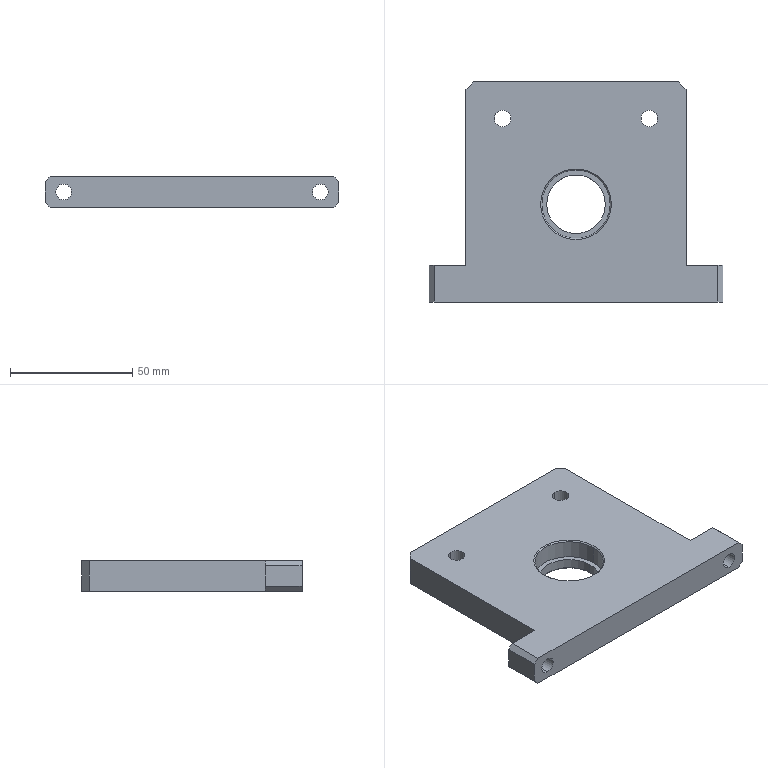Part | SolidWorks | features ICE 4, Chamfer 3, HoleWzd 2, Extrusion 1 | 1 solid | 33 faces | box 120 x 90 x 12.5 mm | volume 97757 mm3 | plane 17 | cylinder 12 | cone 4 | commonest cylinder face diameters 6.5 x4 6.8 x4 24 x2 28 x2
STEP:
#1=CARTESIAN_POINT('',(97.5,0.,-9.5));
#2=VERTEX_POINT('',#1);
#3=CARTESIAN_POINT('',(97.5,0.,-3.));
#4=VERTEX_POINT('',#3);
#5=CARTESIAN_POINT('',(97.5,0.,-6.25));
#6=DIRECTION('',(0.,1.,0.));
#7=DIRECTION('',(0.,0.,1.));
#8=AXIS2_PLACEMENT_3D('',#5,#6,#7);
#9=CIRCLE('',#8,3.25);
#10=EDGE_CURVE('',#2,#4,#9,.T.);
#11=ORIENTED_EDGE('',*,*,#10,.F.);
#12=CARTESIAN_POINT('',(97.5,15.,-9.5));
#13=VERTEX_POINT('',#12);
#14=CARTESIAN_POINT('',(97.5,15.,-9.5));
#15=DIRECTION('',(0.,1.,0.));
#16=VECTOR('',#15,1000.);
#17=LINE('',#14,#16);
#18=EDGE_CURVE('',#2,#13,#17,.T.);
#19=ORIENTED_EDGE('',*,*,#18,.T.);
#20=CARTESIAN_POINT('',(97.5,15.,-3.));
#21=VERTEX_POINT('',#20);
#22=CARTESIAN_POINT('',(97.5,15.,-6.25));
#23=DIRECTION('',(0.,1.,0.));
#24=DIRECTION('',(0.,0.,1.));
#25=AXIS2_PLACEMENT_3D('',#22,#23,#24);
#26=CIRCLE('',#25,3.25);
#27=EDGE_CURVE('',#13,#21,#26,.T.);
#28=ORIENTED_EDGE('',*,*,#27,.T.);
#29=CARTESIAN_POINT('',(97.5,15.,-3.));
#30=DIRECTION('',(0.,1.,0.));
#31=VECTOR('',#30,1000.);
#32=LINE('',#29,#31);
#33=EDGE_CURVE('',#4,#21,#32,.T.);
#34=ORIENTED_EDGE('',*,*,#33,.F.);
#35=EDGE_LOOP('',(#11,#19,#28,#34));
#36=FACE_OUTER_BOUND('',#35,.T.);
#37=CARTESIAN_POINT('',(97.5,15.,-6.25));
#38=DIRECTION('',(0.,1.,0.));
#39=DIRECTION('',(0.,0.,1.));
#40=AXIS2_PLACEMENT_3D('',#37,#38,#39);
#41=CYLINDRICAL_SURFACE('',#40,3.25);
#42=ADVANCED_FACE('',(#36),#41,.F.);
#43=CARTESIAN_POINT('',(-7.5,0.,-9.5));
#44=VERTEX_POINT('',#43);
#45=CARTESIAN_POINT('',(-7.5,0.,-3.));
#46=VERTEX_POINT('',#45);
#47=CARTESIAN_POINT('',(-7.5,0.,-6.25));
#48=DIRECTION('',(0.,1.,0.));
#49=DIRECTION('',(0.,0.,1.));
#50=AXIS2_PLACEMENT_3D('',#47,#48,#49);
#51=CIRCLE('',#50,3.25);
#52=EDGE_CURVE('',#44,#46,#51,.T.);
#53=ORIENTED_EDGE('',*,*,#52,.F.);
#54=CARTESIAN_POINT('',(-7.5,15.,-9.5));
#55=VERTEX_POINT('',#54);
#56=CARTESIAN_POINT('',(-7.5,15.,-9.5));
#57=DIRECTION('',(0.,1.,0.));
#58=VECTOR('',#57,1000.);
#59=LINE('',#56,#58);
#60=EDGE_CURVE('',#44,#55,#59,.T.);
#61=ORIENTED_EDGE('',*,*,#60,.T.);
#62=CARTESIAN_POINT('',(-7.5,15.,-3.));
#63=VERTEX_POINT('',#62);
#64=CARTESIAN_POINT('',(-7.5,15.,-6.25));
#65=DIRECTION('',(0.,1.,0.));
#66=DIRECTION('',(0.,0.,1.));
#67=AXIS2_PLACEMENT_3D('',#64,#65,#66);
#68=CIRCLE('',#67,3.25);
#69=EDGE_CURVE('',#55,#63,#68,.T.);
#70=ORIENTED_EDGE('',*,*,#69,.T.);
#71=CARTESIAN_POINT('',(-7.5,15.,-3.));
#72=DIRECTION('',(0.,1.,0.));
#73=VECTOR('',#72,1000.);
#74=LINE('',#71,#73);
#75=EDGE_CURVE('',#46,#63,#74,.T.);
#76=ORIENTED_EDGE('',*,*,#75,.F.);
#77=EDGE_LOOP('',(#53,#61,#70,#76));
#78=FACE_OUTER_BOUND('',#77,.T.);
#79=CARTESIAN_POINT('',(-7.5,15.,-6.25));
#80=DIRECTION('',(0.,1.,0.));
#81=DIRECTION('',(0.,0.,1.));
#82=AXIS2_PLACEMENT_3D('',#79,#80,#81);
#83=CYLINDRICAL_SURFACE('',#82,3.25);
#84=ADVANCED_FACE('',(#78),#83,.F.);
#85=CARTESIAN_POINT('',(31.,40.,-0.5));
#86=VERTEX_POINT('',#85);
#87=CARTESIAN_POINT('',(59.,40.,-0.5));
#88=VERTEX_POINT('',#87);
#89=CARTESIAN_POINT('',(45.,40.,-0.5));
#90=DIRECTION('',(0.,0.,1.));
#91=DIRECTION('',(-1.,0.,0.));
#92=AXIS2_PLACEMENT_3D('',#89,#90,#91);
#93=CIRCLE('',#92,14.);
#94=EDGE_CURVE('',#86,#88,#93,.T.);
#95=ORIENTED_EDGE('',*,*,#94,.F.);
#96=CARTESIAN_POINT('',(30.5,40.,0.));
#97=VERTEX_POINT('',#96);
#98=CARTESIAN_POINT('',(31.,40.,-0.5));
#99=DIRECTION('',(-0.7071,0.,0.7071));
#100=VECTOR('',#99,1000.);
#101=LINE('',#98,#100);
#102=EDGE_CURVE('',#86,#97,#101,.T.);
#103=ORIENTED_EDGE('',*,*,#102,.T.);
#104=CARTESIAN_POINT('',(59.5,40.,0.));
#105=VERTEX_POINT('',#104);
#106=CARTESIAN_POINT('',(45.,40.,0.));
#107=DIRECTION('',(0.,0.,-1.));
#108=DIRECTION('',(-1.,0.,0.));
#109=AXIS2_PLACEMENT_3D('',#106,#107,#108);
#110=CIRCLE('',#109,14.5);
#111=EDGE_CURVE('',#105,#97,#110,.T.);
#112=ORIENTED_EDGE('',*,*,#111,.F.);
#113=CARTESIAN_POINT('',(59.,40.,-0.5));
#114=DIRECTION('',(0.7071,0.,0.7071));
#115=VECTOR('',#114,1000.);
#116=LINE('',#113,#115);
#117=EDGE_CURVE('',#88,#105,#116,.T.);
#118=ORIENTED_EDGE('',*,*,#117,.F.);
#119=EDGE_LOOP('',(#95,#103,#112,#118));
#120=FACE_OUTER_BOUND('',#119,.T.);
#121=CARTESIAN_POINT('',(45.,40.,-0.5));
#122=DIRECTION('',(0.,0.,1.));
#123=DIRECTION('',(1.,0.,0.));
#124=AXIS2_PLACEMENT_3D('',#121,#122,#123);
#125=CONICAL_SURFACE('',#124,14.,0.7854);
#126=ADVANCED_FACE('',(#120),#125,.F.);
#127=CARTESIAN_POINT('',(57.,40.,-12.));
#128=VERTEX_POINT('',#127);
#129=CARTESIAN_POINT('',(33.,40.,-12.));
#130=VERTEX_POINT('',#129);
#131=CARTESIAN_POINT('',(45.,40.,-12.));
#132=DIRECTION('',(0.,0.,-1.));
#133=DIRECTION('',(1.,0.,0.));
#134=AXIS2_PLACEMENT_3D('',#131,#132,#133);
#135=CIRCLE('',#134,12.);
#136=EDGE_CURVE('',#128,#130,#135,.T.);
#137=ORIENTED_EDGE('',*,*,#136,.F.);
#138=CARTESIAN_POINT('',(57.5,40.,-12.5));
#139=VERTEX_POINT('',#138);
#140=CARTESIAN_POINT('',(57.5,40.,-12.5));
#141=DIRECTION('',(0.7071,0.,-0.7071));
#142=VECTOR('',#141,1000.);
#143=LINE('',#140,#142);
#144=EDGE_CURVE('',#128,#139,#143,.T.);
#145=ORIENTED_EDGE('',*,*,#144,.T.);
#146=CARTESIAN_POINT('',(32.5,40.,-12.5));
#147=VERTEX_POINT('',#146);
#148=CARTESIAN_POINT('',(45.,40.,-12.5));
#149=DIRECTION('',(0.,0.,1.));
#150=DIRECTION('',(0.,-1.,0.));
#151=AXIS2_PLACEMENT_3D('',#148,#149,#150);
#152=CIRCLE('',#151,12.5);
#153=EDGE_CURVE('',#147,#139,#152,.T.);
#154=ORIENTED_EDGE('',*,*,#153,.F.);
#155=CARTESIAN_POINT('',(32.5,40.,-12.5));
#156=DIRECTION('',(-0.7071,0.,-0.7071));
#157=VECTOR('',#156,1000.);
#158=LINE('',#155,#157);
#159=EDGE_CURVE('',#130,#147,#158,.T.);
#160=ORIENTED_EDGE('',*,*,#159,.F.);
#161=EDGE_LOOP('',(#137,#145,#154,#160));
#162=FACE_OUTER_BOUND('',#161,.T.);
#163=CARTESIAN_POINT('',(45.,40.,-12.5));
#164=DIRECTION('',(0.,0.,-1.));
#165=DIRECTION('',(-1.,0.,0.));
#166=AXIS2_PLACEMENT_3D('',#163,#164,#165);
#167=CONICAL_SURFACE('',#166,12.5,0.7854);
#168=ADVANCED_FACE('',(#162),#167,.F.);
#169=ORIENTED_EDGE('',*,*,#136,.T.);
#170=CARTESIAN_POINT('',(33.,40.,-8.));
#171=VERTEX_POINT('',#170);
#172=CARTESIAN_POINT('',(33.,40.,-12.5));
#173=DIRECTION('',(0.,0.,1.));
#174=VECTOR('',#173,1000.);
#175=LINE('',#172,#174);
#176=EDGE_CURVE('',#130,#171,#175,.T.);
#177=ORIENTED_EDGE('',*,*,#176,.T.);
#178=CARTESIAN_POINT('',(57.,40.,-8.));
#179=VERTEX_POINT('',#178);
#180=CARTESIAN_POINT('',(45.,40.,-8.));
#181=DIRECTION('',(0.,0.,1.));
#182=DIRECTION('',(1.,0.,0.));
#183=AXIS2_PLACEMENT_3D('',#180,#181,#182);
#184=CIRCLE('',#183,12.);
#185=EDGE_CURVE('',#171,#179,#184,.T.);
#186=ORIENTED_EDGE('',*,*,#185,.T.);
#187=CARTESIAN_POINT('',(57.,40.,-12.5));
#188=DIRECTION('',(0.,0.,1.));
#189=VECTOR('',#188,1000.);
#190=LINE('',#187,#189);
#191=EDGE_CURVE('',#128,#179,#190,.T.);
#192=ORIENTED_EDGE('',*,*,#191,.F.);
#193=EDGE_LOOP('',(#169,#177,#186,#192));
#194=FACE_OUTER_BOUND('',#193,.T.);
#195=CARTESIAN_POINT('',(45.,40.,-12.5));
#196=DIRECTION('',(0.,0.,1.));
#197=DIRECTION('',(1.,0.,0.));
#198=AXIS2_PLACEMENT_3D('',#195,#196,#197);
#199=CYLINDRICAL_SURFACE('',#198,12.);
#200=ADVANCED_FACE('',(#194),#199,.F.);
#201=CARTESIAN_POINT('',(31.,40.,-8.));
#202=VERTEX_POINT('',#201);
#203=CARTESIAN_POINT('',(59.,40.,-8.));
#204=VERTEX_POINT('',#203);
#205=CARTESIAN_POINT('',(45.,40.,-8.));
#206=DIRECTION('',(0.,0.,1.));
#207=DIRECTION('',(1.,0.,0.));
#208=AXIS2_PLACEMENT_3D('',#205,#206,#207);
#209=CIRCLE('',#208,14.);
#210=EDGE_CURVE('',#202,#204,#209,.T.);
#211=ORIENTED_EDGE('',*,*,#210,.F.);
#212=CARTESIAN_POINT('',(31.,40.,-8.));
#213=DIRECTION('',(0.,0.,1.));
#214=VECTOR('',#213,1000.);
#215=LINE('',#212,#214);
#216=EDGE_CURVE('',#202,#86,#215,.T.);
#217=ORIENTED_EDGE('',*,*,#216,.T.);
#218=ORIENTED_EDGE('',*,*,#94,.T.);
#219=CARTESIAN_POINT('',(59.,40.,-8.));
#220=DIRECTION('',(0.,0.,1.));
#221=VECTOR('',#220,1000.);
#222=LINE('',#219,#221);
#223=EDGE_CURVE('',#204,#88,#222,.T.);
#224=ORIENTED_EDGE('',*,*,#223,.F.);
#225=EDGE_LOOP('',(#211,#217,#218,#224));
#226=FACE_OUTER_BOUND('',#225,.T.);
#227=CARTESIAN_POINT('',(45.,40.,-8.));
#228=DIRECTION('',(0.,0.,1.));
#229=DIRECTION('',(1.,0.,0.));
#230=AXIS2_PLACEMENT_3D('',#227,#228,#229);
#231=CYLINDRICAL_SURFACE('',#230,14.);
#232=ADVANCED_FACE('',(#226),#231,.F.);
#233=CARTESIAN_POINT('',(15.,71.6,0.));
#234=VERTEX_POINT('',#233);
#235=CARTESIAN_POINT('',(15.,78.4,0.));
#236=VERTEX_POINT('',#235);
#237=CARTESIAN_POINT('',(15.,75.,0.));
#238=DIRECTION('',(0.,0.,-1.));
#239=DIRECTION('',(0.,1.,0.));
#240=AXIS2_PLACEMENT_3D('',#237,#238,#239);
#241=CIRCLE('',#240,3.4);
#242=EDGE_CURVE('',#234,#236,#241,.T.);
#243=ORIENTED_EDGE('',*,*,#242,.F.);
#244=CARTESIAN_POINT('',(15.,71.6,-12.5));
#245=VERTEX_POINT('',#244);
#246=CARTESIAN_POINT('',(15.,71.6,-12.5));
#247=DIRECTION('',(0.,0.,-1.));
#248=VECTOR('',#247,1000.);
#249=LINE('',#246,#248);
#250=EDGE_CURVE('',#234,#245,#249,.T.);
#251=ORIENTED_EDGE('',*,*,#250,.T.);
#252=CARTESIAN_POINT('',(15.,78.4,-12.5));
#253=VERTEX_POINT('',#252);
#254=CARTESIAN_POINT('',(15.,75.,-12.5));
#255=DIRECTION('',(0.,0.,-1.));
#256=DIRECTION('',(0.,1.,0.));
#257=AXIS2_PLACEMENT_3D('',#254,#255,#256);
#258=CIRCLE('',#257,3.4);
#259=EDGE_CURVE('',#245,#253,#258,.T.);
#260=ORIENTED_EDGE('',*,*,#259,.T.);
#261=CARTESIAN_POINT('',(15.,78.4,-12.5));
#262=DIRECTION('',(0.,0.,-1.));
#263=VECTOR('',#262,1000.);
#264=LINE('',#261,#263);
#265=EDGE_CURVE('',#236,#253,#264,.T.);
#266=ORIENTED_EDGE('',*,*,#265,.F.);
#267=EDGE_LOOP('',(#243,#251,#260,#266));
#268=FACE_OUTER_BOUND('',#267,.T.);
#269=CARTESIAN_POINT('',(15.,75.,-12.5));
#270=DIRECTION('',(0.,0.,-1.));
#271=DIRECTION('',(0.,1.,0.));
#272=AXIS2_PLACEMENT_3D('',#269,#270,#271);
#273=CYLINDRICAL_SURFACE('',#272,3.4);
#274=ADVANCED_FACE('',(#268),#273,.F.);
#275=CARTESIAN_POINT('',(75.,71.6,0.));
#276=VERTEX_POINT('',#275);
#277=CARTESIAN_POINT('',(75.,78.4,0.));
#278=VERTEX_POINT('',#277);
#279=CARTESIAN_POINT('',(75.,75.,0.));
#280=DIRECTION('',(0.,0.,-1.));
#281=DIRECTION('',(0.,1.,0.));
#282=AXIS2_PLACEMENT_3D('',#279,#280,#281);
#283=CIRCLE('',#282,3.4);
#284=EDGE_CURVE('',#276,#278,#283,.T.);
#285=ORIENTED_EDGE('',*,*,#284,.F.);
#286=CARTESIAN_POINT('',(75.,71.6,-12.5));
#287=VERTEX_POINT('',#286);
#288=CARTESIAN_POINT('',(75.,71.6,-12.5));
#289=DIRECTION('',(0.,0.,-1.));
#290=VECTOR('',#289,1000.);
#291=LINE('',#288,#290);
#292=EDGE_CURVE('',#276,#287,#291,.T.);
#293=ORIENTED_EDGE('',*,*,#292,.T.);
#294=CARTESIAN_POINT('',(75.,78.4,-12.5));
#295=VERTEX_POINT('',#294);
#296=CARTESIAN_POINT('',(75.,75.,-12.5));
#297=DIRECTION('',(0.,0.,-1.));
#298=DIRECTION('',(0.,1.,0.));
#299=AXIS2_PLACEMENT_3D('',#296,#297,#298);
#300=CIRCLE('',#299,3.4);
#301=EDGE_CURVE('',#287,#295,#300,.T.);
#302=ORIENTED_EDGE('',*,*,#301,.T.);
#303=CARTESIAN_POINT('',(75.,78.4,-12.5));
#304=DIRECTION('',(0.,0.,-1.));
#305=VECTOR('',#304,1000.);
#306=LINE('',#303,#305);
#307=EDGE_CURVE('',#278,#295,#306,.T.);
#308=ORIENTED_EDGE('',*,*,#307,.F.);
#309=EDGE_LOOP('',(#285,#293,#302,#308));
#310=FACE_OUTER_BOUND('',#309,.T.);
#311=CARTESIAN_POINT('',(75.,75.,-12.5));
#312=DIRECTION('',(0.,0.,-1.));
#313=DIRECTION('',(0.,1.,0.));
#314=AXIS2_PLACEMENT_3D('',#311,#312,#313);
#315=CYLINDRICAL_SURFACE('',#314,3.4);
#316=ADVANCED_FACE('',(#310),#315,.F.);
#317=CARTESIAN_POINT('',(90.,15.,-12.5));
#318=VERTEX_POINT('',#317);
#319=CARTESIAN_POINT('',(90.,15.,0.));
#320=VERTEX_POINT('',#319);
#321=CARTESIAN_POINT('',(90.,15.,0.));
#322=DIRECTION('',(0.,0.,1.));
#323=VECTOR('',#322,1000.);
#324=LINE('',#321,#323);
#325=EDGE_CURVE('',#318,#320,#324,.T.);
#326=ORIENTED_EDGE('',*,*,#325,.F.);
#327=CARTESIAN_POINT('',(90.,87.,-12.5));
#328=VERTEX_POINT('',#327);
#329=CARTESIAN_POINT('',(90.,90.,-12.5));
#330=DIRECTION('',(0.,1.,0.));
#331=VECTOR('',#330,1000.);
#332=LINE('',#329,#331);
#333=EDGE_CURVE('',#318,#328,#332,.T.);
#334=ORIENTED_EDGE('',*,*,#333,.T.);
#335=CARTESIAN_POINT('',(90.,87.,0.));
#336=VERTEX_POINT('',#335);
#337=CARTESIAN_POINT('',(90.,87.,0.));
#338=DIRECTION('',(0.,0.,1.));
#339=VECTOR('',#338,1000.);
#340=LINE('',#337,#339);
#341=EDGE_CURVE('',#328,#336,#340,.T.);
#342=ORIENTED_EDGE('',*,*,#341,.T.);
#343=CARTESIAN_POINT('',(90.,0.,0.));
#344=DIRECTION('',(0.,-1.,0.));
#345=VECTOR('',#344,1000.);
#346=LINE('',#343,#345);
#347=EDGE_CURVE('',#336,#320,#346,.T.);
#348=ORIENTED_EDGE('',*,*,#347,.T.);
#349=EDGE_LOOP('',(#326,#334,#342,#348));
#350=FACE_OUTER_BOUND('',#349,.T.);
#351=CARTESIAN_POINT('',(90.,0.,0.));
#352=DIRECTION('',(-1.,0.,0.));
#353=DIRECTION('',(0.,0.,1.));
#354=AXIS2_PLACEMENT_3D('',#351,#352,#353);
#355=PLANE('',#354);
#356=ADVANCED_FACE('',(#350),#355,.F.);
#357=CARTESIAN_POINT('',(97.5,0.,-6.25));
#358=DIRECTION('',(0.,1.,0.));
#359=DIRECTION('',(0.,0.,1.));
#360=AXIS2_PLACEMENT_3D('',#357,#358,#359);
#361=CIRCLE('',#360,3.25);
#362=EDGE_CURVE('',#4,#2,#361,.T.);
#363=ORIENTED_EDGE('',*,*,#362,.T.);
#364=ORIENTED_EDGE('',*,*,#10,.T.);
#365=EDGE_LOOP('',(#363,#364));
#366=FACE_BOUND('',#365,.T.);
#367=CARTESIAN_POINT('',(-7.5,0.,-6.25));
#368=DIRECTION('',(0.,1.,0.));
#369=DIRECTION('',(0.,0.,1.));
#370=AXIS2_PLACEMENT_3D('',#367,#368,#369);
#371=CIRCLE('',#370,3.25);
#372=EDGE_CURVE('',#46,#44,#371,.T.);
#373=ORIENTED_EDGE('',*,*,#372,.T.);
#374=ORIENTED_EDGE('',*,*,#52,.T.);
#375=EDGE_LOOP('',(#373,#374));
#376=FACE_BOUND('',#375,.T.);
#377=CARTESIAN_POINT('',(105.,0.,-2.));
#378=VERTEX_POINT('',#377);
#379=CARTESIAN_POINT('',(105.,0.,-10.5));
#380=VERTEX_POINT('',#379);
#381=CARTESIAN_POINT('',(105.,0.,0.));
#382=DIRECTION('',(0.,0.,-1.));
#383=VECTOR('',#382,1000.);
#384=LINE('',#381,#383);
#385=EDGE_CURVE('',#378,#380,#384,.T.);
#386=ORIENTED_EDGE('',*,*,#385,.F.);
#387=CARTESIAN_POINT('',(103.,0.,0.));
#388=VERTEX_POINT('',#387);
#389=CARTESIAN_POINT('',(105.,0.,-2.));
#390=DIRECTION('',(-0.7071,0.,0.7071));
#391=VECTOR('',#390,1000.);
#392=LINE('',#389,#391);
#393=EDGE_CURVE('',#378,#388,#392,.T.);
#394=ORIENTED_EDGE('',*,*,#393,.T.);
#395=CARTESIAN_POINT('',(-13.,0.,0.));
#396=VERTEX_POINT('',#395);
#397=CARTESIAN_POINT('',(90.,0.,0.));
#398=DIRECTION('',(-1.,0.,0.));
#399=VECTOR('',#398,1000.);
#400=LINE('',#397,#399);
#401=EDGE_CURVE('',#388,#396,#400,.T.);
#402=ORIENTED_EDGE('',*,*,#401,.T.);
#403=CARTESIAN_POINT('',(-15.,0.,-2.));
#404=VERTEX_POINT('',#403);
#405=CARTESIAN_POINT('',(-15.,0.,-2.));
#406=DIRECTION('',(-0.7071,0.,-0.7071));
#407=VECTOR('',#406,1000.);
#408=LINE('',#405,#407);
#409=EDGE_CURVE('',#396,#404,#408,.T.);
#410=ORIENTED_EDGE('',*,*,#409,.T.);
#411=CARTESIAN_POINT('',(-15.,0.,-10.5));
#412=VERTEX_POINT('',#411);
#413=CARTESIAN_POINT('',(-15.,0.,-12.5));
#414=DIRECTION('',(0.,0.,1.));
#415=VECTOR('',#414,1000.);
#416=LINE('',#413,#415);
#417=EDGE_CURVE('',#412,#404,#416,.T.);
#418=ORIENTED_EDGE('',*,*,#417,.F.);
#419=CARTESIAN_POINT('',(-13.,0.,-12.5));
#420=VERTEX_POINT('',#419);
#421=CARTESIAN_POINT('',(-15.,0.,-10.5));
#422=DIRECTION('',(0.7071,0.,-0.7071));
#423=VECTOR('',#422,1000.);
#424=LINE('',#421,#423);
#425=EDGE_CURVE('',#412,#420,#424,.T.);
#426=ORIENTED_EDGE('',*,*,#425,.T.);
#427=CARTESIAN_POINT('',(103.,0.,-12.5));
#428=VERTEX_POINT('',#427);
#429=CARTESIAN_POINT('',(90.,0.,-12.5));
#430=DIRECTION('',(-1.,0.,0.));
#431=VECTOR('',#430,1000.);
#432=LINE('',#429,#431);
#433=EDGE_CURVE('',#428,#420,#432,.T.);
#434=ORIENTED_EDGE('',*,*,#433,.F.);
#435=CARTESIAN_POINT('',(105.,0.,-10.5));
#436=DIRECTION('',(0.7071,0.,0.7071));
#437=VECTOR('',#436,1000.);
#438=LINE('',#435,#437);
#439=EDGE_CURVE('',#428,#380,#438,.T.);
#440=ORIENTED_EDGE('',*,*,#439,.T.);
#441=EDGE_LOOP('',(#386,#394,#402,#410,#418,#426,#434,#440));
#442=FACE_OUTER_BOUND('',#441,.T.);
#443=CARTESIAN_POINT('',(90.,0.,-12.5));
#444=DIRECTION('',(0.,1.,0.));
#445=DIRECTION('',(0.,0.,1.));
#446=AXIS2_PLACEMENT_3D('',#443,#444,#445);
#447=PLANE('',#446);
#448=ADVANCED_FACE('',(#366,#376,#442),#447,.F.);
#449=ORIENTED_EDGE('',*,*,#153,.T.);
#450=CARTESIAN_POINT('',(45.,40.,-12.5));
#451=DIRECTION('',(0.,0.,1.));
#452=DIRECTION('',(0.,-1.,0.));
#453=AXIS2_PLACEMENT_3D('',#450,#451,#452);
#454=CIRCLE('',#453,12.5);
#455=EDGE_CURVE('',#139,#147,#454,.T.);
#456=ORIENTED_EDGE('',*,*,#455,.T.);
#457=EDGE_LOOP('',(#449,#456));
#458=FACE_BOUND('',#457,.T.);
#459=CARTESIAN_POINT('',(15.,75.,-12.5));
#460=DIRECTION('',(0.,0.,-1.));
#461=DIRECTION('',(0.,1.,0.));
#462=AXIS2_PLACEMENT_3D('',#459,#460,#461);
#463=CIRCLE('',#462,3.4);
#464=EDGE_CURVE('',#253,#245,#463,.T.);
#465=ORIENTED_EDGE('',*,*,#464,.F.);
#466=ORIENTED_EDGE('',*,*,#259,.F.);
#467=EDGE_LOOP('',(#465,#466));
#468=FACE_BOUND('',#467,.T.);
#469=CARTESIAN_POINT('',(75.,75.,-12.5));
#470=DIRECTION('',(0.,0.,-1.));
#471=DIRECTION('',(0.,1.,0.));
#472=AXIS2_PLACEMENT_3D('',#469,#470,#471);
#473=CIRCLE('',#472,3.4);
#474=EDGE_CURVE('',#295,#287,#473,.T.);
#475=ORIENTED_EDGE('',*,*,#474,.F.);
#476=ORIENTED_EDGE('',*,*,#301,.F.);
#477=EDGE_LOOP('',(#475,#476));
#478=FACE_BOUND('',#477,.T.);
#479=ORIENTED_EDGE('',*,*,#433,.T.);
#480=CARTESIAN_POINT('',(-13.,15.,-12.5));
#481=VERTEX_POINT('',#480);
#482=CARTESIAN_POINT('',(-13.,15.,-12.5));
#483=DIRECTION('',(0.,1.,0.));
#484=VECTOR('',#483,1000.);
#485=LINE('',#482,#484);
#486=EDGE_CURVE('',#420,#481,#485,.T.);
#487=ORIENTED_EDGE('',*,*,#486,.T.);
#488=CARTESIAN_POINT('',(0.,15.,-12.5));
#489=VERTEX_POINT('',#488);
#490=CARTESIAN_POINT('',(-15.,15.,-12.5));
#491=DIRECTION('',(1.,0.,0.));
#492=VECTOR('',#491,1000.);
#493=LINE('',#490,#492);
#494=EDGE_CURVE('',#481,#489,#493,.T.);
#495=ORIENTED_EDGE('',*,*,#494,.T.);
#496=CARTESIAN_POINT('',(0.,87.,-12.5));
#497=VERTEX_POINT('',#496);
#498=CARTESIAN_POINT('',(0.,90.,-12.5));
#499=DIRECTION('',(0.,1.,0.));
#500=VECTOR('',#499,1000.);
#501=LINE('',#498,#500);
#502=EDGE_CURVE('',#489,#497,#501,.T.);
#503=ORIENTED_EDGE('',*,*,#502,.T.);
#504=CARTESIAN_POINT('',(3.,90.,-12.5));
#505=VERTEX_POINT('',#504);
#506=CARTESIAN_POINT('',(3.,90.,-12.5));
#507=DIRECTION('',(0.7071,0.7071,0.));
#508=VECTOR('',#507,1000.);
#509=LINE('',#506,#508);
#510=EDGE_CURVE('',#497,#505,#509,.T.);
#511=ORIENTED_EDGE('',*,*,#510,.T.);
#512=CARTESIAN_POINT('',(87.,90.,-12.5));
#513=VERTEX_POINT('',#512);
#514=CARTESIAN_POINT('',(90.,90.,-12.5));
#515=DIRECTION('',(-1.,0.,0.));
#516=VECTOR('',#515,1000.);
#517=LINE('',#514,#516);
#518=EDGE_CURVE('',#513,#505,#517,.T.);
#519=ORIENTED_EDGE('',*,*,#518,.F.);
#520=CARTESIAN_POINT('',(90.,87.,-12.5));
#521=DIRECTION('',(0.7071,-0.7071,0.));
#522=VECTOR('',#521,1000.);
#523=LINE('',#520,#522);
#524=EDGE_CURVE('',#513,#328,#523,.T.);
#525=ORIENTED_EDGE('',*,*,#524,.T.);
#526=ORIENTED_EDGE('',*,*,#333,.F.);
#527=CARTESIAN_POINT('',(103.,15.,-12.5));
#528=VERTEX_POINT('',#527);
#529=CARTESIAN_POINT('',(105.,15.,-12.5));
#530=DIRECTION('',(-1.,0.,0.));
#531=VECTOR('',#530,1000.);
#532=LINE('',#529,#531);
#533=EDGE_CURVE('',#528,#318,#532,.T.);
#534=ORIENTED_EDGE('',*,*,#533,.F.);
#535=CARTESIAN_POINT('',(103.,90.,-12.5));
#536=DIRECTION('',(0.,-1.,0.));
#537=VECTOR('',#536,1000.);
#538=LINE('',#535,#537);
#539=EDGE_CURVE('',#528,#428,#538,.T.);
#540=ORIENTED_EDGE('',*,*,#539,.T.);
#541=EDGE_LOOP('',(#479,#487,#495,#503,#511,#519,#525,#526,#534,#540));
#542=FACE_OUTER_BOUND('',#541,.T.);
#543=CARTESIAN_POINT('',(90.,90.,-12.5));
#544=DIRECTION('',(0.,0.,1.));
#545=DIRECTION('',(0.,-1.,0.));
#546=AXIS2_PLACEMENT_3D('',#543,#544,#545);
#547=PLANE('',#546);
#548=ADVANCED_FACE('',(#458,#468,#478,#542),#547,.F.);
#549=ORIENTED_EDGE('',*,*,#518,.T.);
#550=CARTESIAN_POINT('',(3.,90.,0.));
#551=VERTEX_POINT('',#550);
#552=CARTESIAN_POINT('',(3.,90.,0.));
#553=DIRECTION('',(0.,0.,1.));
#554=VECTOR('',#553,1000.);
#555=LINE('',#552,#554);
#556=EDGE_CURVE('',#505,#551,#555,.T.);
#557=ORIENTED_EDGE('',*,*,#556,.T.);
#558=CARTESIAN_POINT('',(87.,90.,0.));
#559=VERTEX_POINT('',#558);
#560=CARTESIAN_POINT('',(90.,90.,0.));
#561=DIRECTION('',(-1.,0.,0.));
#562=VECTOR('',#561,1000.);
#563=LINE('',#560,#562);
#564=EDGE_CURVE('',#559,#551,#563,.T.);
#565=ORIENTED_EDGE('',*,*,#564,.F.);
#566=CARTESIAN_POINT('',(87.,90.,0.));
#567=DIRECTION('',(0.,0.,-1.));
#568=VECTOR('',#567,1000.);
#569=LINE('',#566,#568);
#570=EDGE_CURVE('',#559,#513,#569,.T.);
#571=ORIENTED_EDGE('',*,*,#570,.T.);
#572=EDGE_LOOP('',(#549,#557,#565,#571));
#573=FACE_OUTER_BOUND('',#572,.T.);
#574=CARTESIAN_POINT('',(90.,90.,0.));
#575=DIRECTION('',(0.,-1.,0.));
#576=DIRECTION('',(0.,0.,-1.));
#577=AXIS2_PLACEMENT_3D('',#574,#575,#576);
#578=PLANE('',#577);
#579=ADVANCED_FACE('',(#573),#578,.F.);
#580=ORIENTED_EDGE('',*,*,#111,.T.);
#581=CARTESIAN_POINT('',(45.,40.,0.));
#582=DIRECTION('',(0.,0.,-1.));
#583=DIRECTION('',(-1.,0.,0.));
#584=AXIS2_PLACEMENT_3D('',#581,#582,#583);
#585=CIRCLE('',#584,14.5);
#586=EDGE_CURVE('',#97,#105,#585,.T.);
#587=ORIENTED_EDGE('',*,*,#586,.T.);
#588=EDGE_LOOP('',(#580,#587));
#589=FACE_BOUND('',#588,.T.);
#590=CARTESIAN_POINT('',(15.,75.,0.));
#591=DIRECTION('',(0.,0.,-1.));
#592=DIRECTION('',(0.,1.,0.));
#593=AXIS2_PLACEMENT_3D('',#590,#591,#592);
#594=CIRCLE('',#593,3.4);
#595=EDGE_CURVE('',#236,#234,#594,.T.);
#596=ORIENTED_EDGE('',*,*,#595,.T.);
#597=ORIENTED_EDGE('',*,*,#242,.T.);
#598=EDGE_LOOP('',(#596,#597));
#599=FACE_BOUND('',#598,.T.);
#600=CARTESIAN_POINT('',(75.,75.,0.));
#601=DIRECTION('',(0.,0.,-1.));
#602=DIRECTION('',(0.,1.,0.));
#603=AXIS2_PLACEMENT_3D('',#600,#601,#602);
#604=CIRCLE('',#603,3.4);
#605=EDGE_CURVE('',#278,#276,#604,.T.);
#606=ORIENTED_EDGE('',*,*,#605,.T.);
#607=ORIENTED_EDGE('',*,*,#284,.T.);
#608=EDGE_LOOP('',(#606,#607));
#609=FACE_BOUND('',#608,.T.);
#610=ORIENTED_EDGE('',*,*,#401,.F.);
#611=CARTESIAN_POINT('',(103.,15.,0.));
#612=VERTEX_POINT('',#611);
#613=CARTESIAN_POINT('',(103.,0.,0.));
#614=DIRECTION('',(0.,1.,0.));
#615=VECTOR('',#614,1000.);
#616=LINE('',#613,#615);
#617=EDGE_CURVE('',#388,#612,#616,.T.);
#618=ORIENTED_EDGE('',*,*,#617,.T.);
#619=CARTESIAN_POINT('',(105.,15.,0.));
#620=DIRECTION('',(-1.,0.,0.));
#621=VECTOR('',#620,1000.);
#622=LINE('',#619,#621);
#623=EDGE_CURVE('',#612,#320,#622,.T.);
#624=ORIENTED_EDGE('',*,*,#623,.T.);
#625=ORIENTED_EDGE('',*,*,#347,.F.);
#626=CARTESIAN_POINT('',(90.,87.,0.));
#627=DIRECTION('',(-0.7071,0.7071,0.));
#628=VECTOR('',#627,1000.);
#629=LINE('',#626,#628);
#630=EDGE_CURVE('',#336,#559,#629,.T.);
#631=ORIENTED_EDGE('',*,*,#630,.T.);
#632=ORIENTED_EDGE('',*,*,#564,.T.);
#633=CARTESIAN_POINT('',(0.,87.,0.));
#634=VERTEX_POINT('',#633);
#635=CARTESIAN_POINT('',(3.,90.,0.));
#636=DIRECTION('',(-0.7071,-0.7071,0.));
#637=VECTOR('',#636,1000.);
#638=LINE('',#635,#637);
#639=EDGE_CURVE('',#551,#634,#638,.T.);
#640=ORIENTED_EDGE('',*,*,#639,.T.);
#641=CARTESIAN_POINT('',(0.,15.,0.));
#642=VERTEX_POINT('',#641);
#643=CARTESIAN_POINT('',(0.,0.,0.));
#644=DIRECTION('',(0.,-1.,0.));
#645=VECTOR('',#644,1000.);
#646=LINE('',#643,#645);
#647=EDGE_CURVE('',#634,#642,#646,.T.);
#648=ORIENTED_EDGE('',*,*,#647,.T.);
#649=CARTESIAN_POINT('',(-13.,15.,0.));
#650=VERTEX_POINT('',#649);
#651=CARTESIAN_POINT('',(-15.,15.,0.));
#652=DIRECTION('',(1.,0.,0.));
#653=VECTOR('',#652,1000.);
#654=LINE('',#651,#653);
#655=EDGE_CURVE('',#650,#642,#654,.T.);
#656=ORIENTED_EDGE('',*,*,#655,.F.);
#657=CARTESIAN_POINT('',(-13.,0.,0.));
#658=DIRECTION('',(0.,-1.,0.));
#659=VECTOR('',#658,1000.);
#660=LINE('',#657,#659);
#661=EDGE_CURVE('',#650,#396,#660,.T.);
#662=ORIENTED_EDGE('',*,*,#661,.T.);
#663=EDGE_LOOP('',(#610,#618,#624,#625,#631,#632,#640,#648,#656,#662));
#664=FACE_OUTER_BOUND('',#663,.T.);
#665=CARTESIAN_POINT('',(90.,0.,0.));
#666=DIRECTION('',(0.,0.,-1.));
#667=DIRECTION('',(-1.,0.,0.));
#668=AXIS2_PLACEMENT_3D('',#665,#666,#667);
#669=PLANE('',#668);
#670=ADVANCED_FACE('',(#589,#599,#609,#664),#669,.F.);
#671=CARTESIAN_POINT('',(0.,15.,-12.5));
#672=DIRECTION('',(0.,0.,-1.));
#673=VECTOR('',#672,1000.);
#674=LINE('',#671,#673);
#675=EDGE_CURVE('',#642,#489,#674,.T.);
#676=ORIENTED_EDGE('',*,*,#675,.F.);
#677=ORIENTED_EDGE('',*,*,#647,.F.);
#678=CARTESIAN_POINT('',(0.,87.,-12.5));
#679=DIRECTION('',(0.,0.,-1.));
#680=VECTOR('',#679,1000.);
#681=LINE('',#678,#680);
#682=EDGE_CURVE('',#634,#497,#681,.T.);
#683=ORIENTED_EDGE('',*,*,#682,.T.);
#684=ORIENTED_EDGE('',*,*,#502,.F.);
#685=EDGE_LOOP('',(#676,#677,#683,#684));
#686=FACE_OUTER_BOUND('',#685,.T.);
#687=CARTESIAN_POINT('',(0.,0.,0.));
#688=DIRECTION('',(-1.,0.,0.));
#689=DIRECTION('',(0.,0.,1.));
#690=AXIS2_PLACEMENT_3D('',#687,#688,#689);
#691=PLANE('',#690);
#692=ADVANCED_FACE('',(#686),#691,.T.);
#693=ORIENTED_EDGE('',*,*,#510,.F.);
#694=ORIENTED_EDGE('',*,*,#682,.F.);
#695=ORIENTED_EDGE('',*,*,#639,.F.);
#696=ORIENTED_EDGE('',*,*,#556,.F.);
#697=EDGE_LOOP('',(#693,#694,#695,#696));
#698=FACE_OUTER_BOUND('',#697,.T.);
#699=CARTESIAN_POINT('',(3.,90.,0.));
#700=DIRECTION('',(-0.7071,0.7071,0.));
#701=DIRECTION('',(0.,0.,-1.));
#702=AXIS2_PLACEMENT_3D('',#699,#700,#701);
#703=PLANE('',#702);
#704=ADVANCED_FACE('',(#698),#703,.T.);
#705=ORIENTED_EDGE('',*,*,#524,.F.);
#706=ORIENTED_EDGE('',*,*,#570,.F.);
#707=ORIENTED_EDGE('',*,*,#630,.F.);
#708=ORIENTED_EDGE('',*,*,#341,.F.);
#709=EDGE_LOOP('',(#705,#706,#707,#708));
#710=FACE_OUTER_BOUND('',#709,.T.);
#711=CARTESIAN_POINT('',(90.,87.,0.));
#712=DIRECTION('',(-0.7071,-0.7071,0.));
#713=DIRECTION('',(0.,0.,1.));
#714=AXIS2_PLACEMENT_3D('',#711,#712,#713);
#715=PLANE('',#714);
#716=ADVANCED_FACE('',(#710),#715,.F.);
#717=ORIENTED_EDGE('',*,*,#292,.F.);
#718=ORIENTED_EDGE('',*,*,#605,.F.);
#719=ORIENTED_EDGE('',*,*,#307,.T.);
#720=ORIENTED_EDGE('',*,*,#474,.T.);
#721=EDGE_LOOP('',(#717,#718,#719,#720));
#722=FACE_OUTER_BOUND('',#721,.T.);
#723=CARTESIAN_POINT('',(75.,75.,-12.5));
#724=DIRECTION('',(0.,0.,-1.));
#725=DIRECTION('',(0.,1.,0.));
#726=AXIS2_PLACEMENT_3D('',#723,#724,#725);
#727=CYLINDRICAL_SURFACE('',#726,3.4);
#728=ADVANCED_FACE('',(#722),#727,.F.);
#729=ORIENTED_EDGE('',*,*,#250,.F.);
#730=ORIENTED_EDGE('',*,*,#595,.F.);
#731=ORIENTED_EDGE('',*,*,#265,.T.);
#732=ORIENTED_EDGE('',*,*,#464,.T.);
#733=EDGE_LOOP('',(#729,#730,#731,#732));
#734=FACE_OUTER_BOUND('',#733,.T.);
#735=CARTESIAN_POINT('',(15.,75.,-12.5));
#736=DIRECTION('',(0.,0.,-1.));
#737=DIRECTION('',(0.,1.,0.));
#738=AXIS2_PLACEMENT_3D('',#735,#736,#737);
#739=CYLINDRICAL_SURFACE('',#738,3.4);
#740=ADVANCED_FACE('',(#734),#739,.F.);
#741=ORIENTED_EDGE('',*,*,#216,.F.);
#742=CARTESIAN_POINT('',(45.,40.,-8.));
#743=DIRECTION('',(0.,0.,1.));
#744=DIRECTION('',(1.,0.,0.));
#745=AXIS2_PLACEMENT_3D('',#742,#743,#744);
#746=CIRCLE('',#745,14.);
#747=EDGE_CURVE('',#204,#202,#746,.T.);
#748=ORIENTED_EDGE('',*,*,#747,.F.);
#749=ORIENTED_EDGE('',*,*,#223,.T.);
#750=CARTESIAN_POINT('',(45.,40.,-0.5));
#751=DIRECTION('',(0.,0.,1.));
#752=DIRECTION('',(-1.,0.,0.));
#753=AXIS2_PLACEMENT_3D('',#750,#751,#752);
#754=CIRCLE('',#753,14.);
#755=EDGE_CURVE('',#88,#86,#754,.T.);
#756=ORIENTED_EDGE('',*,*,#755,.T.);
#757=EDGE_LOOP('',(#741,#748,#749,#756));
#758=FACE_OUTER_BOUND('',#757,.T.);
#759=CARTESIAN_POINT('',(45.,40.,-8.));
#760=DIRECTION('',(0.,0.,1.));
#761=DIRECTION('',(1.,0.,0.));
#762=AXIS2_PLACEMENT_3D('',#759,#760,#761);
#763=CYLINDRICAL_SURFACE('',#762,14.);
#764=ADVANCED_FACE('',(#758),#763,.F.);
#765=CARTESIAN_POINT('',(45.,40.,-8.));
#766=DIRECTION('',(0.,0.,1.));
#767=DIRECTION('',(1.,0.,0.));
#768=AXIS2_PLACEMENT_3D('',#765,#766,#767);
#769=CIRCLE('',#768,12.);
#770=EDGE_CURVE('',#179,#171,#769,.T.);
#771=ORIENTED_EDGE('',*,*,#770,.F.);
#772=ORIENTED_EDGE('',*,*,#185,.F.);
#773=EDGE_LOOP('',(#771,#772));
#774=FACE_BOUND('',#773,.T.);
#775=ORIENTED_EDGE('',*,*,#747,.T.);
#776=ORIENTED_EDGE('',*,*,#210,.T.);
#777=EDGE_LOOP('',(#775,#776));
#778=FACE_OUTER_BOUND('',#777,.T.);
#779=CARTESIAN_POINT('',(45.,40.,-8.));
#780=DIRECTION('',(0.,0.,1.));
#781=DIRECTION('',(1.,0.,0.));
#782=AXIS2_PLACEMENT_3D('',#779,#780,#781);
#783=PLANE('',#782);
#784=ADVANCED_FACE('',(#774,#778),#783,.T.);
#785=ORIENTED_EDGE('',*,*,#176,.F.);
#786=CARTESIAN_POINT('',(45.,40.,-12.));
#787=DIRECTION('',(0.,0.,-1.));
#788=DIRECTION('',(1.,0.,0.));
#789=AXIS2_PLACEMENT_3D('',#786,#787,#788);
#790=CIRCLE('',#789,12.);
#791=EDGE_CURVE('',#130,#128,#790,.T.);
#792=ORIENTED_EDGE('',*,*,#791,.T.);
#793=ORIENTED_EDGE('',*,*,#191,.T.);
#794=ORIENTED_EDGE('',*,*,#770,.T.);
#795=EDGE_LOOP('',(#785,#792,#793,#794));
#796=FACE_OUTER_BOUND('',#795,.T.);
#797=CARTESIAN_POINT('',(45.,40.,-12.5));
#798=DIRECTION('',(0.,0.,1.));
#799=DIRECTION('',(1.,0.,0.));
#800=AXIS2_PLACEMENT_3D('',#797,#798,#799);
#801=CYLINDRICAL_SURFACE('',#800,12.);
#802=ADVANCED_FACE('',(#796),#801,.F.);
#803=ORIENTED_EDGE('',*,*,#144,.F.);
#804=ORIENTED_EDGE('',*,*,#791,.F.);
#805=ORIENTED_EDGE('',*,*,#159,.T.);
#806=ORIENTED_EDGE('',*,*,#455,.F.);
#807=EDGE_LOOP('',(#803,#804,#805,#806));
#808=FACE_OUTER_BOUND('',#807,.T.);
#809=CARTESIAN_POINT('',(45.,40.,-12.5));
#810=DIRECTION('',(0.,0.,-1.));
#811=DIRECTION('',(-1.,0.,0.));
#812=AXIS2_PLACEMENT_3D('',#809,#810,#811);
#813=CONICAL_SURFACE('',#812,12.5,0.7854);
#814=ADVANCED_FACE('',(#808),#813,.F.);
#815=ORIENTED_EDGE('',*,*,#102,.F.);
#816=ORIENTED_EDGE('',*,*,#755,.F.);
#817=ORIENTED_EDGE('',*,*,#117,.T.);
#818=ORIENTED_EDGE('',*,*,#586,.F.);
#819=EDGE_LOOP('',(#815,#816,#817,#818));
#820=FACE_OUTER_BOUND('',#819,.T.);
#821=CARTESIAN_POINT('',(45.,40.,-0.5));
#822=DIRECTION('',(0.,0.,1.));
#823=DIRECTION('',(1.,0.,0.));
#824=AXIS2_PLACEMENT_3D('',#821,#822,#823);
#825=CONICAL_SURFACE('',#824,14.,0.7854);
#826=ADVANCED_FACE('',(#820),#825,.F.);
#827=CARTESIAN_POINT('',(97.5,15.,-6.25));
#828=DIRECTION('',(0.,1.,0.));
#829=DIRECTION('',(0.,0.,1.));
#830=AXIS2_PLACEMENT_3D('',#827,#828,#829);
#831=CIRCLE('',#830,3.25);
#832=EDGE_CURVE('',#21,#13,#831,.T.);
#833=ORIENTED_EDGE('',*,*,#832,.F.);
#834=ORIENTED_EDGE('',*,*,#27,.F.);
#835=EDGE_LOOP('',(#833,#834));
#836=FACE_BOUND('',#835,.T.);
#837=ORIENTED_EDGE('',*,*,#623,.F.);
#838=CARTESIAN_POINT('',(105.,15.,-2.));
#839=VERTEX_POINT('',#838);
#840=CARTESIAN_POINT('',(105.,15.,-2.));
#841=DIRECTION('',(0.7071,0.,-0.7071));
#842=VECTOR('',#841,1000.);
#843=LINE('',#840,#842);
#844=EDGE_CURVE('',#612,#839,#843,.T.);
#845=ORIENTED_EDGE('',*,*,#844,.T.);
#846=CARTESIAN_POINT('',(105.,15.,-10.5));
#847=VERTEX_POINT('',#846);
#848=CARTESIAN_POINT('',(105.,15.,0.));
#849=DIRECTION('',(0.,0.,1.));
#850=VECTOR('',#849,1000.);
#851=LINE('',#848,#850);
#852=EDGE_CURVE('',#847,#839,#851,.T.);
#853=ORIENTED_EDGE('',*,*,#852,.F.);
#854=CARTESIAN_POINT('',(105.,15.,-10.5));
#855=DIRECTION('',(-0.7071,0.,-0.7071));
#856=VECTOR('',#855,1000.);
#857=LINE('',#854,#856);
#858=EDGE_CURVE('',#847,#528,#857,.T.);
#859=ORIENTED_EDGE('',*,*,#858,.T.);
#860=ORIENTED_EDGE('',*,*,#533,.T.);
#861=ORIENTED_EDGE('',*,*,#325,.T.);
#862=EDGE_LOOP('',(#837,#845,#853,#859,#860,#861));
#863=FACE_OUTER_BOUND('',#862,.T.);
#864=CARTESIAN_POINT('',(105.,15.,0.));
#865=DIRECTION('',(0.,-1.,0.));
#866=DIRECTION('',(0.,0.,-1.));
#867=AXIS2_PLACEMENT_3D('',#864,#865,#866);
#868=PLANE('',#867);
#869=ADVANCED_FACE('',(#836,#863),#868,.F.);
#870=ORIENTED_EDGE('',*,*,#852,.T.);
#871=CARTESIAN_POINT('',(105.,0.,-2.));
#872=DIRECTION('',(0.,-1.,0.));
#873=VECTOR('',#872,1000.);
#874=LINE('',#871,#873);
#875=EDGE_CURVE('',#839,#378,#874,.T.);
#876=ORIENTED_EDGE('',*,*,#875,.T.);
#877=ORIENTED_EDGE('',*,*,#385,.T.);
#878=CARTESIAN_POINT('',(105.,0.,-10.5));
#879=DIRECTION('',(0.,1.,0.));
#880=VECTOR('',#879,1000.);
#881=LINE('',#878,#880);
#882=EDGE_CURVE('',#380,#847,#881,.T.);
#883=ORIENTED_EDGE('',*,*,#882,.T.);
#884=EDGE_LOOP('',(#870,#876,#877,#883));
#885=FACE_OUTER_BOUND('',#884,.T.);
#886=CARTESIAN_POINT('',(105.,0.,0.));
#887=DIRECTION('',(-1.,0.,0.));
#888=DIRECTION('',(0.,0.,1.));
#889=AXIS2_PLACEMENT_3D('',#886,#887,#888);
#890=PLANE('',#889);
#891=ADVANCED_FACE('',(#885),#890,.F.);
#892=CARTESIAN_POINT('',(-7.5,15.,-6.25));
#893=DIRECTION('',(0.,1.,0.));
#894=DIRECTION('',(0.,0.,1.));
#895=AXIS2_PLACEMENT_3D('',#892,#893,#894);
#896=CIRCLE('',#895,3.25);
#897=EDGE_CURVE('',#63,#55,#896,.T.);
#898=ORIENTED_EDGE('',*,*,#897,.F.);
#899=ORIENTED_EDGE('',*,*,#69,.F.);
#900=EDGE_LOOP('',(#898,#899));
#901=FACE_BOUND('',#900,.T.);
#902=CARTESIAN_POINT('',(-15.,15.,-2.));
#903=VERTEX_POINT('',#902);
#904=CARTESIAN_POINT('',(-15.,15.,-10.5));
#905=VERTEX_POINT('',#904);
#906=CARTESIAN_POINT('',(-15.,15.,-12.5));
#907=DIRECTION('',(0.,0.,-1.));
#908=VECTOR('',#907,1000.);
#909=LINE('',#906,#908);
#910=EDGE_CURVE('',#903,#905,#909,.T.);
#911=ORIENTED_EDGE('',*,*,#910,.F.);
#912=CARTESIAN_POINT('',(-15.,15.,-2.));
#913=DIRECTION('',(0.7071,0.,0.7071));
#914=VECTOR('',#913,1000.);
#915=LINE('',#912,#914);
#916=EDGE_CURVE('',#903,#650,#915,.T.);
#917=ORIENTED_EDGE('',*,*,#916,.T.);
#918=ORIENTED_EDGE('',*,*,#655,.T.);
#919=ORIENTED_EDGE('',*,*,#675,.T.);
#920=ORIENTED_EDGE('',*,*,#494,.F.);
#921=CARTESIAN_POINT('',(-15.,15.,-10.5));
#922=DIRECTION('',(-0.7071,0.,0.7071));
#923=VECTOR('',#922,1000.);
#924=LINE('',#921,#923);
#925=EDGE_CURVE('',#481,#905,#924,.T.);
#926=ORIENTED_EDGE('',*,*,#925,.T.);
#927=EDGE_LOOP('',(#911,#917,#918,#919,#920,#926));
#928=FACE_OUTER_BOUND('',#927,.T.);
#929=CARTESIAN_POINT('',(-15.,15.,-12.5));
#930=DIRECTION('',(0.,-1.,0.));
#931=DIRECTION('',(0.,0.,-1.));
#932=AXIS2_PLACEMENT_3D('',#929,#930,#931);
#933=PLANE('',#932);
#934=ADVANCED_FACE('',(#901,#928),#933,.F.);
#935=ORIENTED_EDGE('',*,*,#417,.T.);
#936=CARTESIAN_POINT('',(-15.,15.,-2.));
#937=DIRECTION('',(0.,1.,0.));
#938=VECTOR('',#937,1000.);
#939=LINE('',#936,#938);
#940=EDGE_CURVE('',#404,#903,#939,.T.);
#941=ORIENTED_EDGE('',*,*,#940,.T.);
#942=ORIENTED_EDGE('',*,*,#910,.T.);
#943=CARTESIAN_POINT('',(-15.,0.,-10.5));
#944=DIRECTION('',(0.,-1.,0.));
#945=VECTOR('',#944,1000.);
#946=LINE('',#943,#945);
#947=EDGE_CURVE('',#905,#412,#946,.T.);
#948=ORIENTED_EDGE('',*,*,#947,.T.);
#949=EDGE_LOOP('',(#935,#941,#942,#948));
#950=FACE_OUTER_BOUND('',#949,.T.);
#951=CARTESIAN_POINT('',(-15.,0.,0.));
#952=DIRECTION('',(-1.,0.,0.));
#953=DIRECTION('',(0.,0.,1.));
#954=AXIS2_PLACEMENT_3D('',#951,#952,#953);
#955=PLANE('',#954);
#956=ADVANCED_FACE('',(#950),#955,.T.);
#957=ORIENTED_EDGE('',*,*,#844,.F.);
#958=ORIENTED_EDGE('',*,*,#617,.F.);
#959=ORIENTED_EDGE('',*,*,#393,.F.);
#960=ORIENTED_EDGE('',*,*,#875,.F.);
#961=EDGE_LOOP('',(#957,#958,#959,#960));
#962=FACE_OUTER_BOUND('',#961,.T.);
#963=CARTESIAN_POINT('',(105.,0.,-2.));
#964=DIRECTION('',(-0.7071,0.,-0.7071));
#965=DIRECTION('',(0.,-1.,0.));
#966=AXIS2_PLACEMENT_3D('',#963,#964,#965);
#967=PLANE('',#966);
#968=ADVANCED_FACE('',(#962),#967,.F.);
#969=ORIENTED_EDGE('',*,*,#409,.F.);
#970=ORIENTED_EDGE('',*,*,#661,.F.);
#971=ORIENTED_EDGE('',*,*,#916,.F.);
#972=ORIENTED_EDGE('',*,*,#940,.F.);
#973=EDGE_LOOP('',(#969,#970,#971,#972));
#974=FACE_OUTER_BOUND('',#973,.T.);
#975=CARTESIAN_POINT('',(-15.,0.,-2.));
#976=DIRECTION('',(-0.7071,0.,0.7071));
#977=DIRECTION('',(0.,-1.,0.));
#978=AXIS2_PLACEMENT_3D('',#975,#976,#977);
#979=PLANE('',#978);
#980=ADVANCED_FACE('',(#974),#979,.T.);
#981=ORIENTED_EDGE('',*,*,#925,.F.);
#982=ORIENTED_EDGE('',*,*,#486,.F.);
#983=ORIENTED_EDGE('',*,*,#425,.F.);
#984=ORIENTED_EDGE('',*,*,#947,.F.);
#985=EDGE_LOOP('',(#981,#982,#983,#984));
#986=FACE_OUTER_BOUND('',#985,.T.);
#987=CARTESIAN_POINT('',(-15.,0.,-10.5));
#988=DIRECTION('',(-0.7071,0.,-0.7071));
#989=DIRECTION('',(0.,1.,0.));
#990=AXIS2_PLACEMENT_3D('',#987,#988,#989);
#991=PLANE('',#990);
#992=ADVANCED_FACE('',(#986),#991,.T.);
#993=ORIENTED_EDGE('',*,*,#439,.F.);
#994=ORIENTED_EDGE('',*,*,#539,.F.);
#995=ORIENTED_EDGE('',*,*,#858,.F.);
#996=ORIENTED_EDGE('',*,*,#882,.F.);
#997=EDGE_LOOP('',(#993,#994,#995,#996));
#998=FACE_OUTER_BOUND('',#997,.T.);
#999=CARTESIAN_POINT('',(105.,0.,-10.5));
#1000=DIRECTION('',(-0.7071,0.,0.7071));
#1001=DIRECTION('',(0.,1.,0.));
#1002=AXIS2_PLACEMENT_3D('',#999,#1000,#1001);
#1003=PLANE('',#1002);
#1004=ADVANCED_FACE('',(#998),#1003,.F.);
#1005=ORIENTED_EDGE('',*,*,#60,.F.);
#1006=ORIENTED_EDGE('',*,*,#372,.F.);
#1007=ORIENTED_EDGE('',*,*,#75,.T.);
#1008=ORIENTED_EDGE('',*,*,#897,.T.);
#1009=EDGE_LOOP('',(#1005,#1006,#1007,#1008));
#1010=FACE_OUTER_BOUND('',#1009,.T.);
#1011=CARTESIAN_POINT('',(-7.5,15.,-6.25));
#1012=DIRECTION('',(0.,1.,0.));
#1013=DIRECTION('',(0.,0.,1.));
#1014=AXIS2_PLACEMENT_3D('',#1011,#1012,#1013);
#1015=CYLINDRICAL_SURFACE('',#1014,3.25);
#1016=ADVANCED_FACE('',(#1010),#1015,.F.);
#1017=ORIENTED_EDGE('',*,*,#18,.F.);
#1018=ORIENTED_EDGE('',*,*,#362,.F.);
#1019=ORIENTED_EDGE('',*,*,#33,.T.);
#1020=ORIENTED_EDGE('',*,*,#832,.T.);
#1021=EDGE_LOOP('',(#1017,#1018,#1019,#1020));
#1022=FACE_OUTER_BOUND('',#1021,.T.);
#1023=CARTESIAN_POINT('',(97.5,15.,-6.25));
#1024=DIRECTION('',(0.,1.,0.));
#1025=DIRECTION('',(0.,0.,1.));
#1026=AXIS2_PLACEMENT_3D('',#1023,#1024,#1025);
#1027=CYLINDRICAL_SURFACE('',#1026,3.25);
#1028=ADVANCED_FACE('',(#1022),#1027,.F.);
#1029=CLOSED_SHELL('',(#42,#84,#126,#168,#200,#232,#274,#316,#356,#448,#548,#579,#670,#692,#704,#716,#728,#740,#764,#784,#802,#814,#826,#869,#891,#934,#956,#968,#980,#992,#1004,#1016,#1028));
#1030=MANIFOLD_SOLID_BREP('',#1029);
#1031=CARTESIAN_POINT('',(0.,0.,0.));
#1032=DIRECTION('',(0.,0.,1.));
#1033=DIRECTION('',(1.,0.,0.));
#1034=AXIS2_PLACEMENT_3D('',#1031,#1032,#1033);
#1035=(LENGTH_UNIT()NAMED_UNIT(*)SI_UNIT(.MILLI.,.METRE.));
#1036=UNCERTAINTY_MEASURE_WITH_UNIT(LENGTH_MEASURE(0.00001),#1035,'','');
#1037=(NAMED_UNIT(*)PLANE_ANGLE_UNIT()SI_UNIT($,.RADIAN.));
#1038=(NAMED_UNIT(*)SI_UNIT($,.STERADIAN.)SOLID_ANGLE_UNIT());
#1039=(GEOMETRIC_REPRESENTATION_CONTEXT(3)GLOBAL_UNCERTAINTY_ASSIGNED_CONTEXT((#1036))GLOBAL_UNIT_ASSIGNED_CONTEXT((#1035,#1037,#1038))REPRESENTATION_CONTEXT('',''));
#1040=ADVANCED_BREP_SHAPE_REPRESENTATION('',(#1030,#1034),#1039);